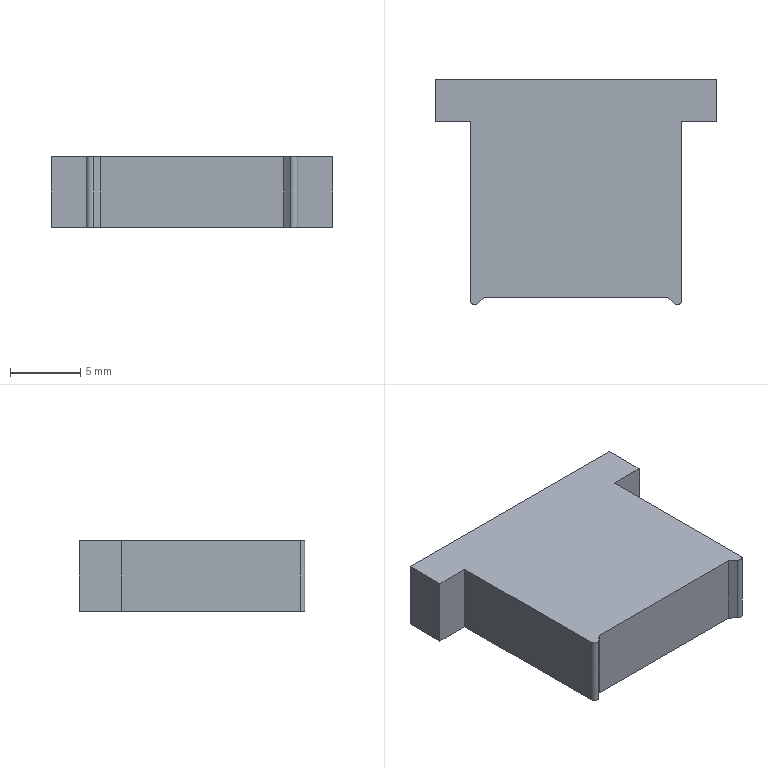Part | STEP file | iron shell positioning insert-1 | 1 solid | 17 faces | box 20 x 16.011 x 5 mm | volume 1177 mm3 | plane 11 | cylinder 6 | commonest cylinder face diameters 0.6 x2 4.5 x2 20.6 x2
STEP:
#1=CARTESIAN_POINT('',(0.,0.,0.));
#2=DIRECTION('',(0.,0.,1.));
#3=DIRECTION('',(1.,0.,0.));
#4=AXIS2_PLACEMENT_3D('',#1,#2,#3);
#5=CARTESIAN_POINT('',(-2.25,5.75,2.5));
#6=VERTEX_POINT('',#5);
#7=CARTESIAN_POINT('',(-2.25,9.75,2.5));
#8=VERTEX_POINT('',#7);
#9=CARTESIAN_POINT('',(-2.25,5.75,2.5));
#10=DIRECTION('',(0.,1.,0.));
#11=VECTOR('',#10,1.);
#12=LINE('',#9,#11);
#13=CARTESIAN_POINT('',(0.,5.75,2.5));
#14=DIRECTION('',(0.,1.,0.));
#15=DIRECTION('',(-1.,0.,0.));
#16=AXIS2_PLACEMENT_3D('',#13,#14,#15);
#17=CYLINDRICAL_SURFACE('',#16,2.25);
#18=CARTESIAN_POINT('',(6.283,0.));
#19=DIRECTION('',(0.,1.));
#20=VECTOR('',#19,1.);
#21=LINE('',#18,#20);
#22=(GEOMETRIC_REPRESENTATION_CONTEXT(2)PARAMETRIC_REPRESENTATION_CONTEXT()REPRESENTATION_CONTEXT('',''));
#23=DEFINITIONAL_REPRESENTATION('',(#21),#22);
#24=PCURVE('',#17,#23);
#25=CARTESIAN_POINT('',(0.,5.75,2.5));
#26=DIRECTION('',(0.,1.,0.));
#27=DIRECTION('',(-1.,0.,0.));
#28=AXIS2_PLACEMENT_3D('',#25,#26,#27);
#29=CYLINDRICAL_SURFACE('',#28,2.25);
#30=CARTESIAN_POINT('',(0.,0.));
#31=DIRECTION('',(0.,1.));
#32=VECTOR('',#31,1.);
#33=LINE('',#30,#32);
#34=(GEOMETRIC_REPRESENTATION_CONTEXT(2)PARAMETRIC_REPRESENTATION_CONTEXT()REPRESENTATION_CONTEXT('',''));
#35=DEFINITIONAL_REPRESENTATION('',(#33),#34);
#36=PCURVE('',#29,#35);
#37=SURFACE_CURVE('',#12,(#24,#36),.PCURVE_S1.);
#38=EDGE_CURVE('',#6,#8,#37,.T.);
#39=ORIENTED_EDGE('',*,*,#38,.T.);
#40=CARTESIAN_POINT('',(2.25,9.75,2.5));
#41=VERTEX_POINT('',#40);
#42=CARTESIAN_POINT('',(0.,9.75,2.5));
#43=DIRECTION('',(0.,1.,0.));
#44=DIRECTION('',(-1.,0.,0.));
#45=AXIS2_PLACEMENT_3D('',#42,#43,#44);
#46=CIRCLE('',#45,2.25);
#47=CARTESIAN_POINT('',(0.,4.));
#48=DIRECTION('',(1.,0.));
#49=VECTOR('',#48,1.);
#50=LINE('',#47,#49);
#51=(GEOMETRIC_REPRESENTATION_CONTEXT(2)PARAMETRIC_REPRESENTATION_CONTEXT()REPRESENTATION_CONTEXT('',''));
#52=DEFINITIONAL_REPRESENTATION('',(#50),#51);
#53=PCURVE('',#17,#52);
#54=CARTESIAN_POINT('',(-10.,9.75,5.));
#55=DIRECTION('',(0.,-1.,0.));
#56=DIRECTION('',(0.,0.,-1.));
#57=AXIS2_PLACEMENT_3D('',#54,#55,#56);
#58=PLANE('',#57);
#59=CARTESIAN_POINT('',(2.5,7.75));
#60=CARTESIAN_POINT('',(-1.397,7.75));
#61=CARTESIAN_POINT('',(0.5514,11.125));
#62=CARTESIAN_POINT('',(2.5,14.5));
#63=CARTESIAN_POINT('',(4.449,11.125));
#64=CARTESIAN_POINT('',(6.397,7.75));
#65=CARTESIAN_POINT('',(2.5,7.75));
#66=(BOUNDED_CURVE()B_SPLINE_CURVE(2,(#59,#60,#61,#62,#63,#64,#65),.UNSPECIFIED.,.T.,.F.)B_SPLINE_CURVE_WITH_KNOTS((1,2,2,2,2,1),(-2.094,0.,2.094,4.189,6.283,8.378),.UNSPECIFIED.)CURVE()GEOMETRIC_REPRESENTATION_ITEM()RATIONAL_B_SPLINE_CURVE((1.,0.5,1.,0.5,1.,0.5,1.))REPRESENTATION_ITEM(''));
#67=(GEOMETRIC_REPRESENTATION_CONTEXT(2)PARAMETRIC_REPRESENTATION_CONTEXT()REPRESENTATION_CONTEXT('',''));
#68=DEFINITIONAL_REPRESENTATION('',(#66),#67);
#69=PCURVE('',#58,#68);
#70=SURFACE_CURVE('',#46,(#53,#69),.PCURVE_S1.);
#71=EDGE_CURVE('',#41,#8,#70,.T.);
#72=ORIENTED_EDGE('',*,*,#71,.F.);
#73=CARTESIAN_POINT('',(2.25,5.75,2.5));
#74=VERTEX_POINT('',#73);
#75=CARTESIAN_POINT('',(2.25,5.75,2.5));
#76=DIRECTION('',(0.,1.,0.));
#77=VECTOR('',#76,1.);
#78=LINE('',#75,#77);
#79=CARTESIAN_POINT('',(3.142,0.));
#80=DIRECTION('',(0.,1.));
#81=VECTOR('',#80,1.);
#82=LINE('',#79,#81);
#83=(GEOMETRIC_REPRESENTATION_CONTEXT(2)PARAMETRIC_REPRESENTATION_CONTEXT()REPRESENTATION_CONTEXT('',''));
#84=DEFINITIONAL_REPRESENTATION('',(#82),#83);
#85=PCURVE('',#17,#84);
#86=CARTESIAN_POINT('',(3.142,0.));
#87=DIRECTION('',(0.,1.));
#88=VECTOR('',#87,1.);
#89=LINE('',#86,#88);
#90=(GEOMETRIC_REPRESENTATION_CONTEXT(2)PARAMETRIC_REPRESENTATION_CONTEXT()REPRESENTATION_CONTEXT('',''));
#91=DEFINITIONAL_REPRESENTATION('',(#89),#90);
#92=PCURVE('',#29,#91);
#93=SURFACE_CURVE('',#78,(#85,#92),.PCURVE_S1.);
#94=EDGE_CURVE('',#74,#41,#93,.T.);
#95=ORIENTED_EDGE('',*,*,#94,.F.);
#96=CARTESIAN_POINT('',(0.,5.75,2.5));
#97=DIRECTION('',(0.,1.,0.));
#98=DIRECTION('',(-1.,0.,0.));
#99=AXIS2_PLACEMENT_3D('',#96,#97,#98);
#100=CIRCLE('',#99,2.25);
#101=CARTESIAN_POINT('',(0.,0.));
#102=DIRECTION('',(1.,0.));
#103=VECTOR('',#102,1.);
#104=LINE('',#101,#103);
#105=(GEOMETRIC_REPRESENTATION_CONTEXT(2)PARAMETRIC_REPRESENTATION_CONTEXT()REPRESENTATION_CONTEXT('',''));
#106=DEFINITIONAL_REPRESENTATION('',(#104),#105);
#107=PCURVE('',#17,#106);
#108=CARTESIAN_POINT('',(0.,5.75,2.5));
#109=DIRECTION('',(0.,1.,0.));
#110=DIRECTION('',(-1.,0.,0.));
#111=AXIS2_PLACEMENT_3D('',#108,#109,#110);
#112=PLANE('',#111);
#113=CARTESIAN_POINT('',(0.,0.));
#114=DIRECTION('',(1.,0.));
#115=AXIS2_PLACEMENT_2D('',#113,#114);
#116=CIRCLE('',#115,2.25);
#117=(GEOMETRIC_REPRESENTATION_CONTEXT(2)PARAMETRIC_REPRESENTATION_CONTEXT()REPRESENTATION_CONTEXT('',''));
#118=DEFINITIONAL_REPRESENTATION('',(#116),#117);
#119=PCURVE('',#112,#118);
#120=SURFACE_CURVE('',#100,(#107,#119),.PCURVE_S1.);
#121=EDGE_CURVE('',#74,#6,#120,.T.);
#122=ORIENTED_EDGE('',*,*,#121,.T.);
#123=EDGE_LOOP('',(#39,#72,#95,#122));
#124=FACE_BOUND('',#123,.F.);
#125=ADVANCED_FACE('',(#124),#17,.F.);
#126=CARTESIAN_POINT('',(-10.,6.75,0.));
#127=VERTEX_POINT('',#126);
#128=CARTESIAN_POINT('',(-7.5,6.75,0.));
#129=VERTEX_POINT('',#128);
#130=CARTESIAN_POINT('',(-10.,6.75,0.));
#131=DIRECTION('',(1.,0.,0.));
#132=VECTOR('',#131,1.);
#133=LINE('',#130,#132);
#134=CARTESIAN_POINT('',(-10.,6.75,5.));
#135=DIRECTION('',(0.,1.,0.));
#136=DIRECTION('',(-1.,0.,0.));
#137=AXIS2_PLACEMENT_3D('',#134,#135,#136);
#138=PLANE('',#137);
#139=CARTESIAN_POINT('',(0.,-5.));
#140=DIRECTION('',(-1.,0.));
#141=VECTOR('',#140,1.);
#142=LINE('',#139,#141);
#143=(GEOMETRIC_REPRESENTATION_CONTEXT(2)PARAMETRIC_REPRESENTATION_CONTEXT()REPRESENTATION_CONTEXT('',''));
#144=DEFINITIONAL_REPRESENTATION('',(#142),#143);
#145=PCURVE('',#138,#144);
#146=CARTESIAN_POINT('',(-7.2,-5.961,0.));
#147=DIRECTION('',(0.,0.,1.));
#148=DIRECTION('',(1.,0.,0.));
#149=AXIS2_PLACEMENT_3D('',#146,#147,#148);
#150=PLANE('',#149);
#151=CARTESIAN_POINT('',(-2.8,12.711));
#152=DIRECTION('',(1.,0.));
#153=VECTOR('',#152,1.);
#154=LINE('',#151,#153);
#155=(GEOMETRIC_REPRESENTATION_CONTEXT(2)PARAMETRIC_REPRESENTATION_CONTEXT()REPRESENTATION_CONTEXT('',''));
#156=DEFINITIONAL_REPRESENTATION('',(#154),#155);
#157=PCURVE('',#150,#156);
#158=SURFACE_CURVE('',#133,(#145,#157),.PCURVE_S1.);
#159=EDGE_CURVE('',#127,#129,#158,.T.);
#160=ORIENTED_EDGE('',*,*,#159,.T.);
#161=CARTESIAN_POINT('',(-7.5,6.75,5.));
#162=VERTEX_POINT('',#161);
#163=CARTESIAN_POINT('',(-7.5,6.75,5.));
#164=DIRECTION('',(0.,0.,-1.));
#165=VECTOR('',#164,1.);
#166=LINE('',#163,#165);
#167=CARTESIAN_POINT('',(-2.5,0.));
#168=DIRECTION('',(0.,-1.));
#169=VECTOR('',#168,1.);
#170=LINE('',#167,#169);
#171=(GEOMETRIC_REPRESENTATION_CONTEXT(2)PARAMETRIC_REPRESENTATION_CONTEXT()REPRESENTATION_CONTEXT('',''));
#172=DEFINITIONAL_REPRESENTATION('',(#170),#171);
#173=PCURVE('',#138,#172);
#174=CARTESIAN_POINT('',(-7.5,6.75,5.));
#175=DIRECTION('',(1.,0.,0.));
#176=DIRECTION('',(0.,0.,-1.));
#177=AXIS2_PLACEMENT_3D('',#174,#175,#176);
#178=PLANE('',#177);
#179=CARTESIAN_POINT('',(0.,0.));
#180=DIRECTION('',(1.,0.));
#181=VECTOR('',#180,1.);
#182=LINE('',#179,#181);
#183=(GEOMETRIC_REPRESENTATION_CONTEXT(2)PARAMETRIC_REPRESENTATION_CONTEXT()REPRESENTATION_CONTEXT('',''));
#184=DEFINITIONAL_REPRESENTATION('',(#182),#183);
#185=PCURVE('',#178,#184);
#186=SURFACE_CURVE('',#166,(#173,#185),.PCURVE_S1.);
#187=EDGE_CURVE('',#162,#129,#186,.T.);
#188=ORIENTED_EDGE('',*,*,#187,.F.);
#189=CARTESIAN_POINT('',(-10.,6.75,5.));
#190=VERTEX_POINT('',#189);
#191=CARTESIAN_POINT('',(-10.,6.75,5.));
#192=DIRECTION('',(1.,0.,0.));
#193=VECTOR('',#192,1.);
#194=LINE('',#191,#193);
#195=CARTESIAN_POINT('',(0.,0.));
#196=DIRECTION('',(-1.,0.));
#197=VECTOR('',#196,1.);
#198=LINE('',#195,#197);
#199=(GEOMETRIC_REPRESENTATION_CONTEXT(2)PARAMETRIC_REPRESENTATION_CONTEXT()REPRESENTATION_CONTEXT('',''));
#200=DEFINITIONAL_REPRESENTATION('',(#198),#199);
#201=PCURVE('',#138,#200);
#202=CARTESIAN_POINT('',(-7.2,-5.961,5.));
#203=DIRECTION('',(0.,0.,1.));
#204=DIRECTION('',(1.,0.,0.));
#205=AXIS2_PLACEMENT_3D('',#202,#203,#204);
#206=PLANE('',#205);
#207=CARTESIAN_POINT('',(-2.8,12.711));
#208=DIRECTION('',(1.,0.));
#209=VECTOR('',#208,1.);
#210=LINE('',#207,#209);
#211=(GEOMETRIC_REPRESENTATION_CONTEXT(2)PARAMETRIC_REPRESENTATION_CONTEXT()REPRESENTATION_CONTEXT('',''));
#212=DEFINITIONAL_REPRESENTATION('',(#210),#211);
#213=PCURVE('',#206,#212);
#214=SURFACE_CURVE('',#194,(#201,#213),.PCURVE_S1.);
#215=EDGE_CURVE('',#190,#162,#214,.T.);
#216=ORIENTED_EDGE('',*,*,#215,.F.);
#217=CARTESIAN_POINT('',(-10.,6.75,5.));
#218=DIRECTION('',(0.,0.,-1.));
#219=VECTOR('',#218,1.);
#220=LINE('',#217,#219);
#221=CARTESIAN_POINT('',(0.,0.));
#222=DIRECTION('',(0.,-1.));
#223=VECTOR('',#222,1.);
#224=LINE('',#221,#223);
#225=(GEOMETRIC_REPRESENTATION_CONTEXT(2)PARAMETRIC_REPRESENTATION_CONTEXT()REPRESENTATION_CONTEXT('',''));
#226=DEFINITIONAL_REPRESENTATION('',(#224),#225);
#227=PCURVE('',#138,#226);
#228=CARTESIAN_POINT('',(-10.,9.75,5.));
#229=DIRECTION('',(1.,0.,0.));
#230=DIRECTION('',(0.,1.,0.));
#231=AXIS2_PLACEMENT_3D('',#228,#229,#230);
#232=PLANE('',#231);
#233=CARTESIAN_POINT('',(-3.,0.));
#234=DIRECTION('',(0.,-1.));
#235=VECTOR('',#234,1.);
#236=LINE('',#233,#235);
#237=(GEOMETRIC_REPRESENTATION_CONTEXT(2)PARAMETRIC_REPRESENTATION_CONTEXT()REPRESENTATION_CONTEXT('',''));
#238=DEFINITIONAL_REPRESENTATION('',(#236),#237);
#239=PCURVE('',#232,#238);
#240=SURFACE_CURVE('',#220,(#227,#239),.PCURVE_S1.);
#241=EDGE_CURVE('',#190,#127,#240,.T.);
#242=ORIENTED_EDGE('',*,*,#241,.T.);
#243=EDGE_LOOP('',(#160,#188,#216,#242));
#244=FACE_BOUND('',#243,.T.);
#245=ADVANCED_FACE('',(#244),#138,.F.);
#246=CARTESIAN_POINT('',(-7.5,-5.961,0.));
#247=VERTEX_POINT('',#246);
#248=CARTESIAN_POINT('',(-7.5,6.75,0.));
#249=DIRECTION('',(0.,-1.,0.));
#250=VECTOR('',#249,1.);
#251=LINE('',#248,#250);
#252=CARTESIAN_POINT('',(5.,0.));
#253=DIRECTION('',(0.,-1.));
#254=VECTOR('',#253,1.);
#255=LINE('',#252,#254);
#256=(GEOMETRIC_REPRESENTATION_CONTEXT(2)PARAMETRIC_REPRESENTATION_CONTEXT()REPRESENTATION_CONTEXT('',''));
#257=DEFINITIONAL_REPRESENTATION('',(#255),#256);
#258=PCURVE('',#178,#257);
#259=CARTESIAN_POINT('',(-0.3,12.711));
#260=DIRECTION('',(0.,-1.));
#261=VECTOR('',#260,1.);
#262=LINE('',#259,#261);
#263=(GEOMETRIC_REPRESENTATION_CONTEXT(2)PARAMETRIC_REPRESENTATION_CONTEXT()REPRESENTATION_CONTEXT('',''));
#264=DEFINITIONAL_REPRESENTATION('',(#262),#263);
#265=PCURVE('',#150,#264);
#266=SURFACE_CURVE('',#251,(#258,#265),.PCURVE_S1.);
#267=EDGE_CURVE('',#129,#247,#266,.T.);
#268=ORIENTED_EDGE('',*,*,#267,.T.);
#269=CARTESIAN_POINT('',(-7.5,-5.961,5.));
#270=VERTEX_POINT('',#269);
#271=CARTESIAN_POINT('',(-7.5,-5.961,5.));
#272=DIRECTION('',(0.,0.,-1.));
#273=VECTOR('',#272,1.);
#274=LINE('',#271,#273);
#275=CARTESIAN_POINT('',(0.,-12.711));
#276=DIRECTION('',(1.,0.));
#277=VECTOR('',#276,1.);
#278=LINE('',#275,#277);
#279=(GEOMETRIC_REPRESENTATION_CONTEXT(2)PARAMETRIC_REPRESENTATION_CONTEXT()REPRESENTATION_CONTEXT('',''));
#280=DEFINITIONAL_REPRESENTATION('',(#278),#279);
#281=PCURVE('',#178,#280);
#282=CARTESIAN_POINT('',(-7.2,-5.961,5.));
#283=DIRECTION('',(0.,0.,-1.));
#284=DIRECTION('',(-1.,0.,0.));
#285=AXIS2_PLACEMENT_3D('',#282,#283,#284);
#286=CYLINDRICAL_SURFACE('',#285,0.3);
#287=CARTESIAN_POINT('',(6.283,0.));
#288=DIRECTION('',(0.,1.));
#289=VECTOR('',#288,1.);
#290=LINE('',#287,#289);
#291=(GEOMETRIC_REPRESENTATION_CONTEXT(2)PARAMETRIC_REPRESENTATION_CONTEXT()REPRESENTATION_CONTEXT('',''));
#292=DEFINITIONAL_REPRESENTATION('',(#290),#291);
#293=PCURVE('',#286,#292);
#294=SURFACE_CURVE('',#274,(#281,#293),.PCURVE_S1.);
#295=EDGE_CURVE('',#270,#247,#294,.T.);
#296=ORIENTED_EDGE('',*,*,#295,.F.);
#297=CARTESIAN_POINT('',(-7.5,6.75,5.));
#298=DIRECTION('',(0.,-1.,0.));
#299=VECTOR('',#298,1.);
#300=LINE('',#297,#299);
#301=CARTESIAN_POINT('',(0.,0.));
#302=DIRECTION('',(0.,-1.));
#303=VECTOR('',#302,1.);
#304=LINE('',#301,#303);
#305=(GEOMETRIC_REPRESENTATION_CONTEXT(2)PARAMETRIC_REPRESENTATION_CONTEXT()REPRESENTATION_CONTEXT('',''));
#306=DEFINITIONAL_REPRESENTATION('',(#304),#305);
#307=PCURVE('',#178,#306);
#308=CARTESIAN_POINT('',(-0.3,12.711));
#309=DIRECTION('',(0.,-1.));
#310=VECTOR('',#309,1.);
#311=LINE('',#308,#310);
#312=(GEOMETRIC_REPRESENTATION_CONTEXT(2)PARAMETRIC_REPRESENTATION_CONTEXT()REPRESENTATION_CONTEXT('',''));
#313=DEFINITIONAL_REPRESENTATION('',(#311),#312);
#314=PCURVE('',#206,#313);
#315=SURFACE_CURVE('',#300,(#307,#314),.PCURVE_S1.);
#316=EDGE_CURVE('',#162,#270,#315,.T.);
#317=ORIENTED_EDGE('',*,*,#316,.F.);
#318=ORIENTED_EDGE('',*,*,#187,.T.);
#319=EDGE_LOOP('',(#268,#296,#317,#318));
#320=FACE_BOUND('',#319,.T.);
#321=ADVANCED_FACE('',(#320),#178,.F.);
#322=CARTESIAN_POINT('',(-6.996,-6.181,0.));
#323=VERTEX_POINT('',#322);
#324=CARTESIAN_POINT('',(-7.2,-5.961,0.));
#325=DIRECTION('',(0.,0.,1.));
#326=DIRECTION('',(1.,0.,0.));
#327=AXIS2_PLACEMENT_3D('',#324,#325,#326);
#328=CIRCLE('',#327,0.3);
#329=CARTESIAN_POINT('',(9.425,5.));
#330=DIRECTION('',(-1.,0.));
#331=VECTOR('',#330,1.);
#332=LINE('',#329,#331);
#333=(GEOMETRIC_REPRESENTATION_CONTEXT(2)PARAMETRIC_REPRESENTATION_CONTEXT()REPRESENTATION_CONTEXT('',''));
#334=DEFINITIONAL_REPRESENTATION('',(#332),#333);
#335=PCURVE('',#286,#334);
#336=CARTESIAN_POINT('',(0.,0.));
#337=DIRECTION('',(1.,0.));
#338=AXIS2_PLACEMENT_2D('',#336,#337);
#339=CIRCLE('',#338,0.3);
#340=(GEOMETRIC_REPRESENTATION_CONTEXT(2)PARAMETRIC_REPRESENTATION_CONTEXT()REPRESENTATION_CONTEXT('',''));
#341=DEFINITIONAL_REPRESENTATION('',(#339),#340);
#342=PCURVE('',#150,#341);
#343=SURFACE_CURVE('',#328,(#335,#342),.PCURVE_S1.);
#344=EDGE_CURVE('',#247,#323,#343,.T.);
#345=ORIENTED_EDGE('',*,*,#344,.T.);
#346=CARTESIAN_POINT('',(-6.996,-6.181,5.));
#347=VERTEX_POINT('',#346);
#348=CARTESIAN_POINT('',(-6.996,-6.181,5.));
#349=DIRECTION('',(0.,0.,-1.));
#350=VECTOR('',#349,1.);
#351=LINE('',#348,#350);
#352=CARTESIAN_POINT('',(3.966,0.));
#353=DIRECTION('',(0.,1.));
#354=VECTOR('',#353,1.);
#355=LINE('',#352,#354);
#356=(GEOMETRIC_REPRESENTATION_CONTEXT(2)PARAMETRIC_REPRESENTATION_CONTEXT()REPRESENTATION_CONTEXT('',''));
#357=DEFINITIONAL_REPRESENTATION('',(#355),#356);
#358=PCURVE('',#286,#357);
#359=CARTESIAN_POINT('',(0.,-13.74,5.));
#360=DIRECTION('',(0.,0.,-1.));
#361=DIRECTION('',(-1.,0.,0.));
#362=AXIS2_PLACEMENT_3D('',#359,#360,#361);
#363=CYLINDRICAL_SURFACE('',#362,10.3);
#364=CARTESIAN_POINT('',(0.8241,0.));
#365=DIRECTION('',(0.,1.));
#366=VECTOR('',#365,1.);
#367=LINE('',#364,#366);
#368=(GEOMETRIC_REPRESENTATION_CONTEXT(2)PARAMETRIC_REPRESENTATION_CONTEXT()REPRESENTATION_CONTEXT('',''));
#369=DEFINITIONAL_REPRESENTATION('',(#367),#368);
#370=PCURVE('',#363,#369);
#371=SURFACE_CURVE('',#351,(#358,#370),.PCURVE_S1.);
#372=EDGE_CURVE('',#347,#323,#371,.T.);
#373=ORIENTED_EDGE('',*,*,#372,.F.);
#374=CARTESIAN_POINT('',(-7.2,-5.961,5.));
#375=DIRECTION('',(0.,0.,1.));
#376=DIRECTION('',(1.,0.,0.));
#377=AXIS2_PLACEMENT_3D('',#374,#375,#376);
#378=CIRCLE('',#377,0.3);
#379=CARTESIAN_POINT('',(9.425,0.));
#380=DIRECTION('',(-1.,0.));
#381=VECTOR('',#380,1.);
#382=LINE('',#379,#381);
#383=(GEOMETRIC_REPRESENTATION_CONTEXT(2)PARAMETRIC_REPRESENTATION_CONTEXT()REPRESENTATION_CONTEXT('',''));
#384=DEFINITIONAL_REPRESENTATION('',(#382),#383);
#385=PCURVE('',#286,#384);
#386=CARTESIAN_POINT('',(0.,0.));
#387=DIRECTION('',(1.,0.));
#388=AXIS2_PLACEMENT_2D('',#386,#387);
#389=CIRCLE('',#388,0.3);
#390=(GEOMETRIC_REPRESENTATION_CONTEXT(2)PARAMETRIC_REPRESENTATION_CONTEXT()REPRESENTATION_CONTEXT('',''));
#391=DEFINITIONAL_REPRESENTATION('',(#389),#390);
#392=PCURVE('',#206,#391);
#393=SURFACE_CURVE('',#378,(#385,#392),.PCURVE_S1.);
#394=EDGE_CURVE('',#270,#347,#393,.T.);
#395=ORIENTED_EDGE('',*,*,#394,.F.);
#396=ORIENTED_EDGE('',*,*,#295,.T.);
#397=EDGE_LOOP('',(#345,#373,#395,#396));
#398=FACE_BOUND('',#397,.T.);
#399=ADVANCED_FACE('',(#398),#286,.T.);
#400=ORIENTED_EDGE('',*,*,#372,.F.);
#401=CARTESIAN_POINT('',(-6.5,-5.75,5.));
#402=VERTEX_POINT('',#401);
#403=CARTESIAN_POINT('',(0.,-13.74,5.));
#404=DIRECTION('',(0.,0.,-1.));
#405=DIRECTION('',(1.,0.,0.));
#406=AXIS2_PLACEMENT_3D('',#403,#404,#405);
#407=CIRCLE('',#406,10.3);
#408=CARTESIAN_POINT('',(-3.142,0.));
#409=DIRECTION('',(1.,0.));
#410=VECTOR('',#409,1.);
#411=LINE('',#408,#410);
#412=(GEOMETRIC_REPRESENTATION_CONTEXT(2)PARAMETRIC_REPRESENTATION_CONTEXT()REPRESENTATION_CONTEXT('',''));
#413=DEFINITIONAL_REPRESENTATION('',(#411),#412);
#414=PCURVE('',#363,#413);
#415=CARTESIAN_POINT('',(17.5,-7.779));
#416=CARTESIAN_POINT('',(17.5,-25.62));
#417=CARTESIAN_POINT('',(2.05,-16.7));
#418=CARTESIAN_POINT('',(-13.4,-7.779));
#419=CARTESIAN_POINT('',(2.05,1.141));
#420=CARTESIAN_POINT('',(17.5,10.061));
#421=CARTESIAN_POINT('',(17.5,-7.779));
#422=(BOUNDED_CURVE()B_SPLINE_CURVE(2,(#415,#416,#417,#418,#419,#420,#421),.UNSPECIFIED.,.T.,.F.)B_SPLINE_CURVE_WITH_KNOTS((1,2,2,2,2,1),(-2.094,0.,2.094,4.189,6.283,8.378),.UNSPECIFIED.)CURVE()GEOMETRIC_REPRESENTATION_ITEM()RATIONAL_B_SPLINE_CURVE((1.,0.5,1.,0.5,1.,0.5,1.))REPRESENTATION_ITEM(''));
#423=(GEOMETRIC_REPRESENTATION_CONTEXT(2)PARAMETRIC_REPRESENTATION_CONTEXT()REPRESENTATION_CONTEXT('',''));
#424=DEFINITIONAL_REPRESENTATION('',(#422),#423);
#425=PCURVE('',#206,#424);
#426=SURFACE_CURVE('',#407,(#414,#425),.PCURVE_S1.);
#427=EDGE_CURVE('',#347,#402,#426,.T.);
#428=ORIENTED_EDGE('',*,*,#427,.T.);
#429=CARTESIAN_POINT('',(-6.5,-5.75,0.));
#430=VERTEX_POINT('',#429);
#431=CARTESIAN_POINT('',(-6.5,-5.75,5.));
#432=DIRECTION('',(0.,0.,-1.));
#433=VECTOR('',#432,1.);
#434=LINE('',#431,#433);
#435=CARTESIAN_POINT('',(0.8879,0.));
#436=DIRECTION('',(0.,1.));
#437=VECTOR('',#436,1.);
#438=LINE('',#435,#437);
#439=(GEOMETRIC_REPRESENTATION_CONTEXT(2)PARAMETRIC_REPRESENTATION_CONTEXT()REPRESENTATION_CONTEXT('',''));
#440=DEFINITIONAL_REPRESENTATION('',(#438),#439);
#441=PCURVE('',#363,#440);
#442=CARTESIAN_POINT('',(-6.5,-5.75,5.));
#443=DIRECTION('',(0.,1.,0.));
#444=DIRECTION('',(0.,0.,1.));
#445=AXIS2_PLACEMENT_3D('',#442,#443,#444);
#446=PLANE('',#445);
#447=CARTESIAN_POINT('',(0.,0.));
#448=DIRECTION('',(-1.,0.));
#449=VECTOR('',#448,1.);
#450=LINE('',#447,#449);
#451=(GEOMETRIC_REPRESENTATION_CONTEXT(2)PARAMETRIC_REPRESENTATION_CONTEXT()REPRESENTATION_CONTEXT('',''));
#452=DEFINITIONAL_REPRESENTATION('',(#450),#451);
#453=PCURVE('',#446,#452);
#454=SURFACE_CURVE('',#434,(#441,#453),.PCURVE_S1.);
#455=EDGE_CURVE('',#402,#430,#454,.T.);
#456=ORIENTED_EDGE('',*,*,#455,.T.);
#457=CARTESIAN_POINT('',(0.,-13.74,0.));
#458=DIRECTION('',(0.,0.,-1.));
#459=DIRECTION('',(1.,0.,0.));
#460=AXIS2_PLACEMENT_3D('',#457,#458,#459);
#461=CIRCLE('',#460,10.3);
#462=CARTESIAN_POINT('',(-3.142,5.));
#463=DIRECTION('',(1.,0.));
#464=VECTOR('',#463,1.);
#465=LINE('',#462,#464);
#466=(GEOMETRIC_REPRESENTATION_CONTEXT(2)PARAMETRIC_REPRESENTATION_CONTEXT()REPRESENTATION_CONTEXT('',''));
#467=DEFINITIONAL_REPRESENTATION('',(#465),#466);
#468=PCURVE('',#363,#467);
#469=CARTESIAN_POINT('',(17.5,-7.779));
#470=CARTESIAN_POINT('',(17.5,-25.62));
#471=CARTESIAN_POINT('',(2.05,-16.7));
#472=CARTESIAN_POINT('',(-13.4,-7.779));
#473=CARTESIAN_POINT('',(2.05,1.141));
#474=CARTESIAN_POINT('',(17.5,10.061));
#475=CARTESIAN_POINT('',(17.5,-7.779));
#476=(BOUNDED_CURVE()B_SPLINE_CURVE(2,(#469,#470,#471,#472,#473,#474,#475),.UNSPECIFIED.,.T.,.F.)B_SPLINE_CURVE_WITH_KNOTS((1,2,2,2,2,1),(-2.094,0.,2.094,4.189,6.283,8.378),.UNSPECIFIED.)CURVE()GEOMETRIC_REPRESENTATION_ITEM()RATIONAL_B_SPLINE_CURVE((1.,0.5,1.,0.5,1.,0.5,1.))REPRESENTATION_ITEM(''));
#477=(GEOMETRIC_REPRESENTATION_CONTEXT(2)PARAMETRIC_REPRESENTATION_CONTEXT()REPRESENTATION_CONTEXT('',''));
#478=DEFINITIONAL_REPRESENTATION('',(#476),#477);
#479=PCURVE('',#150,#478);
#480=SURFACE_CURVE('',#461,(#468,#479),.PCURVE_S1.);
#481=EDGE_CURVE('',#323,#430,#480,.T.);
#482=ORIENTED_EDGE('',*,*,#481,.F.);
#483=EDGE_LOOP('',(#400,#428,#456,#482));
#484=FACE_BOUND('',#483,.F.);
#485=ADVANCED_FACE('',(#484),#363,.F.);
#486=CARTESIAN_POINT('',(6.5,-5.75,0.));
#487=VERTEX_POINT('',#486);
#488=CARTESIAN_POINT('',(-6.5,-5.75,0.));
#489=DIRECTION('',(1.,0.,0.));
#490=VECTOR('',#489,1.);
#491=LINE('',#488,#490);
#492=CARTESIAN_POINT('',(-5.,0.));
#493=DIRECTION('',(0.,1.));
#494=VECTOR('',#493,1.);
#495=LINE('',#492,#494);
#496=(GEOMETRIC_REPRESENTATION_CONTEXT(2)PARAMETRIC_REPRESENTATION_CONTEXT()REPRESENTATION_CONTEXT('',''));
#497=DEFINITIONAL_REPRESENTATION('',(#495),#496);
#498=PCURVE('',#446,#497);
#499=CARTESIAN_POINT('',(0.7,0.2105));
#500=DIRECTION('',(1.,0.));
#501=VECTOR('',#500,1.);
#502=LINE('',#499,#501);
#503=(GEOMETRIC_REPRESENTATION_CONTEXT(2)PARAMETRIC_REPRESENTATION_CONTEXT()REPRESENTATION_CONTEXT('',''));
#504=DEFINITIONAL_REPRESENTATION('',(#502),#503);
#505=PCURVE('',#150,#504);
#506=SURFACE_CURVE('',#491,(#498,#505),.PCURVE_S1.);
#507=EDGE_CURVE('',#430,#487,#506,.T.);
#508=ORIENTED_EDGE('',*,*,#507,.T.);
#509=CARTESIAN_POINT('',(6.5,-5.75,5.));
#510=VERTEX_POINT('',#509);
#511=CARTESIAN_POINT('',(6.5,-5.75,5.));
#512=DIRECTION('',(0.,0.,-1.));
#513=VECTOR('',#512,1.);
#514=LINE('',#511,#513);
#515=CARTESIAN_POINT('',(0.,13.));
#516=DIRECTION('',(-1.,0.));
#517=VECTOR('',#516,1.);
#518=LINE('',#515,#517);
#519=(GEOMETRIC_REPRESENTATION_CONTEXT(2)PARAMETRIC_REPRESENTATION_CONTEXT()REPRESENTATION_CONTEXT('',''));
#520=DEFINITIONAL_REPRESENTATION('',(#518),#519);
#521=PCURVE('',#446,#520);
#522=CARTESIAN_POINT('',(0.,-13.74,5.));
#523=DIRECTION('',(0.,0.,-1.));
#524=DIRECTION('',(-1.,0.,0.));
#525=AXIS2_PLACEMENT_3D('',#522,#523,#524);
#526=CYLINDRICAL_SURFACE('',#525,10.3);
#527=CARTESIAN_POINT('',(2.254,0.));
#528=DIRECTION('',(0.,1.));
#529=VECTOR('',#528,1.);
#530=LINE('',#527,#529);
#531=(GEOMETRIC_REPRESENTATION_CONTEXT(2)PARAMETRIC_REPRESENTATION_CONTEXT()REPRESENTATION_CONTEXT('',''));
#532=DEFINITIONAL_REPRESENTATION('',(#530),#531);
#533=PCURVE('',#526,#532);
#534=SURFACE_CURVE('',#514,(#521,#533),.PCURVE_S1.);
#535=EDGE_CURVE('',#510,#487,#534,.T.);
#536=ORIENTED_EDGE('',*,*,#535,.F.);
#537=CARTESIAN_POINT('',(-6.5,-5.75,5.));
#538=DIRECTION('',(1.,0.,0.));
#539=VECTOR('',#538,1.);
#540=LINE('',#537,#539);
#541=CARTESIAN_POINT('',(0.,0.));
#542=DIRECTION('',(0.,1.));
#543=VECTOR('',#542,1.);
#544=LINE('',#541,#543);
#545=(GEOMETRIC_REPRESENTATION_CONTEXT(2)PARAMETRIC_REPRESENTATION_CONTEXT()REPRESENTATION_CONTEXT('',''));
#546=DEFINITIONAL_REPRESENTATION('',(#544),#545);
#547=PCURVE('',#446,#546);
#548=CARTESIAN_POINT('',(0.7,0.2105));
#549=DIRECTION('',(1.,0.));
#550=VECTOR('',#549,1.);
#551=LINE('',#548,#550);
#552=(GEOMETRIC_REPRESENTATION_CONTEXT(2)PARAMETRIC_REPRESENTATION_CONTEXT()REPRESENTATION_CONTEXT('',''));
#553=DEFINITIONAL_REPRESENTATION('',(#551),#552);
#554=PCURVE('',#206,#553);
#555=SURFACE_CURVE('',#540,(#547,#554),.PCURVE_S1.);
#556=EDGE_CURVE('',#402,#510,#555,.T.);
#557=ORIENTED_EDGE('',*,*,#556,.F.);
#558=ORIENTED_EDGE('',*,*,#455,.T.);
#559=EDGE_LOOP('',(#508,#536,#557,#558));
#560=FACE_BOUND('',#559,.T.);
#561=ADVANCED_FACE('',(#560),#446,.F.);
#562=ORIENTED_EDGE('',*,*,#535,.F.);
#563=CARTESIAN_POINT('',(6.996,-6.181,5.));
#564=VERTEX_POINT('',#563);
#565=CARTESIAN_POINT('',(0.,-13.74,5.));
#566=DIRECTION('',(0.,0.,-1.));
#567=DIRECTION('',(1.,0.,0.));
#568=AXIS2_PLACEMENT_3D('',#565,#566,#567);
#569=CIRCLE('',#568,10.3);
#570=CARTESIAN_POINT('',(-3.142,0.));
#571=DIRECTION('',(1.,0.));
#572=VECTOR('',#571,1.);
#573=LINE('',#570,#572);
#574=(GEOMETRIC_REPRESENTATION_CONTEXT(2)PARAMETRIC_REPRESENTATION_CONTEXT()REPRESENTATION_CONTEXT('',''));
#575=DEFINITIONAL_REPRESENTATION('',(#573),#574);
#576=PCURVE('',#526,#575);
#577=CARTESIAN_POINT('',(17.5,-7.779));
#578=CARTESIAN_POINT('',(17.5,-25.62));
#579=CARTESIAN_POINT('',(2.05,-16.7));
#580=CARTESIAN_POINT('',(-13.4,-7.779));
#581=CARTESIAN_POINT('',(2.05,1.141));
#582=CARTESIAN_POINT('',(17.5,10.061));
#583=CARTESIAN_POINT('',(17.5,-7.779));
#584=(BOUNDED_CURVE()B_SPLINE_CURVE(2,(#577,#578,#579,#580,#581,#582,#583),.UNSPECIFIED.,.T.,.F.)B_SPLINE_CURVE_WITH_KNOTS((1,2,2,2,2,1),(-2.094,0.,2.094,4.189,6.283,8.378),.UNSPECIFIED.)CURVE()GEOMETRIC_REPRESENTATION_ITEM()RATIONAL_B_SPLINE_CURVE((1.,0.5,1.,0.5,1.,0.5,1.))REPRESENTATION_ITEM(''));
#585=(GEOMETRIC_REPRESENTATION_CONTEXT(2)PARAMETRIC_REPRESENTATION_CONTEXT()REPRESENTATION_CONTEXT('',''));
#586=DEFINITIONAL_REPRESENTATION('',(#584),#585);
#587=PCURVE('',#206,#586);
#588=SURFACE_CURVE('',#569,(#576,#587),.PCURVE_S1.);
#589=EDGE_CURVE('',#510,#564,#588,.T.);
#590=ORIENTED_EDGE('',*,*,#589,.T.);
#591=CARTESIAN_POINT('',(6.996,-6.181,0.));
#592=VERTEX_POINT('',#591);
#593=CARTESIAN_POINT('',(6.996,-6.181,5.));
#594=DIRECTION('',(0.,0.,-1.));
#595=VECTOR('',#594,1.);
#596=LINE('',#593,#595);
#597=CARTESIAN_POINT('',(2.318,0.));
#598=DIRECTION('',(0.,1.));
#599=VECTOR('',#598,1.);
#600=LINE('',#597,#599);
#601=(GEOMETRIC_REPRESENTATION_CONTEXT(2)PARAMETRIC_REPRESENTATION_CONTEXT()REPRESENTATION_CONTEXT('',''));
#602=DEFINITIONAL_REPRESENTATION('',(#600),#601);
#603=PCURVE('',#526,#602);
#604=CARTESIAN_POINT('',(7.2,-5.961,5.));
#605=DIRECTION('',(0.,0.,-1.));
#606=DIRECTION('',(-1.,0.,0.));
#607=AXIS2_PLACEMENT_3D('',#604,#605,#606);
#608=CYLINDRICAL_SURFACE('',#607,0.3);
#609=CARTESIAN_POINT('',(5.459,0.));
#610=DIRECTION('',(0.,1.));
#611=VECTOR('',#610,1.);
#612=LINE('',#609,#611);
#613=(GEOMETRIC_REPRESENTATION_CONTEXT(2)PARAMETRIC_REPRESENTATION_CONTEXT()REPRESENTATION_CONTEXT('',''));
#614=DEFINITIONAL_REPRESENTATION('',(#612),#613);
#615=PCURVE('',#608,#614);
#616=SURFACE_CURVE('',#596,(#603,#615),.PCURVE_S1.);
#617=EDGE_CURVE('',#564,#592,#616,.T.);
#618=ORIENTED_EDGE('',*,*,#617,.T.);
#619=CARTESIAN_POINT('',(0.,-13.74,0.));
#620=DIRECTION('',(0.,0.,-1.));
#621=DIRECTION('',(1.,0.,0.));
#622=AXIS2_PLACEMENT_3D('',#619,#620,#621);
#623=CIRCLE('',#622,10.3);
#624=CARTESIAN_POINT('',(-3.142,5.));
#625=DIRECTION('',(1.,0.));
#626=VECTOR('',#625,1.);
#627=LINE('',#624,#626);
#628=(GEOMETRIC_REPRESENTATION_CONTEXT(2)PARAMETRIC_REPRESENTATION_CONTEXT()REPRESENTATION_CONTEXT('',''));
#629=DEFINITIONAL_REPRESENTATION('',(#627),#628);
#630=PCURVE('',#526,#629);
#631=CARTESIAN_POINT('',(17.5,-7.779));
#632=CARTESIAN_POINT('',(17.5,-25.62));
#633=CARTESIAN_POINT('',(2.05,-16.7));
#634=CARTESIAN_POINT('',(-13.4,-7.779));
#635=CARTESIAN_POINT('',(2.05,1.141));
#636=CARTESIAN_POINT('',(17.5,10.061));
#637=CARTESIAN_POINT('',(17.5,-7.779));
#638=(BOUNDED_CURVE()B_SPLINE_CURVE(2,(#631,#632,#633,#634,#635,#636,#637),.UNSPECIFIED.,.T.,.F.)B_SPLINE_CURVE_WITH_KNOTS((1,2,2,2,2,1),(-2.094,0.,2.094,4.189,6.283,8.378),.UNSPECIFIED.)CURVE()GEOMETRIC_REPRESENTATION_ITEM()RATIONAL_B_SPLINE_CURVE((1.,0.5,1.,0.5,1.,0.5,1.))REPRESENTATION_ITEM(''));
#639=(GEOMETRIC_REPRESENTATION_CONTEXT(2)PARAMETRIC_REPRESENTATION_CONTEXT()REPRESENTATION_CONTEXT('',''));
#640=DEFINITIONAL_REPRESENTATION('',(#638),#639);
#641=PCURVE('',#150,#640);
#642=SURFACE_CURVE('',#623,(#630,#641),.PCURVE_S1.);
#643=EDGE_CURVE('',#487,#592,#642,.T.);
#644=ORIENTED_EDGE('',*,*,#643,.F.);
#645=EDGE_LOOP('',(#562,#590,#618,#644));
#646=FACE_BOUND('',#645,.F.);
#647=ADVANCED_FACE('',(#646),#526,.F.);
#648=CARTESIAN_POINT('',(7.5,-5.961,0.));
#649=VERTEX_POINT('',#648);
#650=CARTESIAN_POINT('',(7.2,-5.961,0.));
#651=DIRECTION('',(0.,0.,1.));
#652=DIRECTION('',(1.,0.,0.));
#653=AXIS2_PLACEMENT_3D('',#650,#651,#652);
#654=CIRCLE('',#653,0.3);
#655=CARTESIAN_POINT('',(9.425,5.));
#656=DIRECTION('',(-1.,0.));
#657=VECTOR('',#656,1.);
#658=LINE('',#655,#657);
#659=(GEOMETRIC_REPRESENTATION_CONTEXT(2)PARAMETRIC_REPRESENTATION_CONTEXT()REPRESENTATION_CONTEXT('',''));
#660=DEFINITIONAL_REPRESENTATION('',(#658),#659);
#661=PCURVE('',#608,#660);
#662=CARTESIAN_POINT('',(14.4,0.));
#663=DIRECTION('',(1.,0.));
#664=AXIS2_PLACEMENT_2D('',#662,#663);
#665=CIRCLE('',#664,0.3);
#666=(GEOMETRIC_REPRESENTATION_CONTEXT(2)PARAMETRIC_REPRESENTATION_CONTEXT()REPRESENTATION_CONTEXT('',''));
#667=DEFINITIONAL_REPRESENTATION('',(#665),#666);
#668=PCURVE('',#150,#667);
#669=SURFACE_CURVE('',#654,(#661,#668),.PCURVE_S1.);
#670=EDGE_CURVE('',#592,#649,#669,.T.);
#671=ORIENTED_EDGE('',*,*,#670,.T.);
#672=CARTESIAN_POINT('',(7.5,-5.961,5.));
#673=VERTEX_POINT('',#672);
#674=CARTESIAN_POINT('',(7.5,-5.961,5.));
#675=DIRECTION('',(0.,0.,-1.));
#676=VECTOR('',#675,1.);
#677=LINE('',#674,#676);
#678=CARTESIAN_POINT('',(3.142,0.));
#679=DIRECTION('',(0.,1.));
#680=VECTOR('',#679,1.);
#681=LINE('',#678,#680);
#682=(GEOMETRIC_REPRESENTATION_CONTEXT(2)PARAMETRIC_REPRESENTATION_CONTEXT()REPRESENTATION_CONTEXT('',''));
#683=DEFINITIONAL_REPRESENTATION('',(#681),#682);
#684=PCURVE('',#608,#683);
#685=CARTESIAN_POINT('',(7.5,6.75,5.));
#686=DIRECTION('',(-1.,0.,0.));
#687=DIRECTION('',(0.,0.,1.));
#688=AXIS2_PLACEMENT_3D('',#685,#686,#687);
#689=PLANE('',#688);
#690=CARTESIAN_POINT('',(0.,-12.711));
#691=DIRECTION('',(-1.,0.));
#692=VECTOR('',#691,1.);
#693=LINE('',#690,#692);
#694=(GEOMETRIC_REPRESENTATION_CONTEXT(2)PARAMETRIC_REPRESENTATION_CONTEXT()REPRESENTATION_CONTEXT('',''));
#695=DEFINITIONAL_REPRESENTATION('',(#693),#694);
#696=PCURVE('',#689,#695);
#697=SURFACE_CURVE('',#677,(#684,#696),.PCURVE_S1.);
#698=EDGE_CURVE('',#673,#649,#697,.T.);
#699=ORIENTED_EDGE('',*,*,#698,.F.);
#700=CARTESIAN_POINT('',(7.2,-5.961,5.));
#701=DIRECTION('',(0.,0.,1.));
#702=DIRECTION('',(1.,0.,0.));
#703=AXIS2_PLACEMENT_3D('',#700,#701,#702);
#704=CIRCLE('',#703,0.3);
#705=CARTESIAN_POINT('',(9.425,0.));
#706=DIRECTION('',(-1.,0.));
#707=VECTOR('',#706,1.);
#708=LINE('',#705,#707);
#709=(GEOMETRIC_REPRESENTATION_CONTEXT(2)PARAMETRIC_REPRESENTATION_CONTEXT()REPRESENTATION_CONTEXT('',''));
#710=DEFINITIONAL_REPRESENTATION('',(#708),#709);
#711=PCURVE('',#608,#710);
#712=CARTESIAN_POINT('',(14.4,0.));
#713=DIRECTION('',(1.,0.));
#714=AXIS2_PLACEMENT_2D('',#712,#713);
#715=CIRCLE('',#714,0.3);
#716=(GEOMETRIC_REPRESENTATION_CONTEXT(2)PARAMETRIC_REPRESENTATION_CONTEXT()REPRESENTATION_CONTEXT('',''));
#717=DEFINITIONAL_REPRESENTATION('',(#715),#716);
#718=PCURVE('',#206,#717);
#719=SURFACE_CURVE('',#704,(#711,#718),.PCURVE_S1.);
#720=EDGE_CURVE('',#564,#673,#719,.T.);
#721=ORIENTED_EDGE('',*,*,#720,.F.);
#722=ORIENTED_EDGE('',*,*,#617,.T.);
#723=EDGE_LOOP('',(#671,#699,#721,#722));
#724=FACE_BOUND('',#723,.T.);
#725=ADVANCED_FACE('',(#724),#608,.T.);
#726=CARTESIAN_POINT('',(7.5,6.75,0.));
#727=VERTEX_POINT('',#726);
#728=CARTESIAN_POINT('',(7.5,6.75,0.));
#729=DIRECTION('',(0.,1.,0.));
#730=VECTOR('',#729,1.);
#731=LINE('',#728,#730);
#732=CARTESIAN_POINT('',(-5.,0.));
#733=DIRECTION('',(0.,1.));
#734=VECTOR('',#733,1.);
#735=LINE('',#732,#734);
#736=(GEOMETRIC_REPRESENTATION_CONTEXT(2)PARAMETRIC_REPRESENTATION_CONTEXT()REPRESENTATION_CONTEXT('',''));
#737=DEFINITIONAL_REPRESENTATION('',(#735),#736);
#738=PCURVE('',#689,#737);
#739=CARTESIAN_POINT('',(14.7,12.711));
#740=DIRECTION('',(0.,1.));
#741=VECTOR('',#740,1.);
#742=LINE('',#739,#741);
#743=(GEOMETRIC_REPRESENTATION_CONTEXT(2)PARAMETRIC_REPRESENTATION_CONTEXT()REPRESENTATION_CONTEXT('',''));
#744=DEFINITIONAL_REPRESENTATION('',(#742),#743);
#745=PCURVE('',#150,#744);
#746=SURFACE_CURVE('',#731,(#738,#745),.PCURVE_S1.);
#747=EDGE_CURVE('',#649,#727,#746,.T.);
#748=ORIENTED_EDGE('',*,*,#747,.T.);
#749=CARTESIAN_POINT('',(7.5,6.75,5.));
#750=VERTEX_POINT('',#749);
#751=CARTESIAN_POINT('',(7.5,6.75,5.));
#752=DIRECTION('',(0.,0.,-1.));
#753=VECTOR('',#752,1.);
#754=LINE('',#751,#753);
#755=CARTESIAN_POINT('',(0.,0.));
#756=DIRECTION('',(-1.,0.));
#757=VECTOR('',#756,1.);
#758=LINE('',#755,#757);
#759=(GEOMETRIC_REPRESENTATION_CONTEXT(2)PARAMETRIC_REPRESENTATION_CONTEXT()REPRESENTATION_CONTEXT('',''));
#760=DEFINITIONAL_REPRESENTATION('',(#758),#759);
#761=PCURVE('',#689,#760);
#762=CARTESIAN_POINT('',(7.5,6.75,5.));
#763=DIRECTION('',(0.,1.,0.));
#764=DIRECTION('',(-1.,0.,0.));
#765=AXIS2_PLACEMENT_3D('',#762,#763,#764);
#766=PLANE('',#765);
#767=CARTESIAN_POINT('',(0.,0.));
#768=DIRECTION('',(0.,-1.));
#769=VECTOR('',#768,1.);
#770=LINE('',#767,#769);
#771=(GEOMETRIC_REPRESENTATION_CONTEXT(2)PARAMETRIC_REPRESENTATION_CONTEXT()REPRESENTATION_CONTEXT('',''));
#772=DEFINITIONAL_REPRESENTATION('',(#770),#771);
#773=PCURVE('',#766,#772);
#774=SURFACE_CURVE('',#754,(#761,#773),.PCURVE_S1.);
#775=EDGE_CURVE('',#750,#727,#774,.T.);
#776=ORIENTED_EDGE('',*,*,#775,.F.);
#777=CARTESIAN_POINT('',(7.5,6.75,5.));
#778=DIRECTION('',(0.,1.,0.));
#779=VECTOR('',#778,1.);
#780=LINE('',#777,#779);
#781=CARTESIAN_POINT('',(0.,0.));
#782=DIRECTION('',(0.,1.));
#783=VECTOR('',#782,1.);
#784=LINE('',#781,#783);
#785=(GEOMETRIC_REPRESENTATION_CONTEXT(2)PARAMETRIC_REPRESENTATION_CONTEXT()REPRESENTATION_CONTEXT('',''));
#786=DEFINITIONAL_REPRESENTATION('',(#784),#785);
#787=PCURVE('',#689,#786);
#788=CARTESIAN_POINT('',(14.7,12.711));
#789=DIRECTION('',(0.,1.));
#790=VECTOR('',#789,1.);
#791=LINE('',#788,#790);
#792=(GEOMETRIC_REPRESENTATION_CONTEXT(2)PARAMETRIC_REPRESENTATION_CONTEXT()REPRESENTATION_CONTEXT('',''));
#793=DEFINITIONAL_REPRESENTATION('',(#791),#792);
#794=PCURVE('',#206,#793);
#795=SURFACE_CURVE('',#780,(#787,#794),.PCURVE_S1.);
#796=EDGE_CURVE('',#673,#750,#795,.T.);
#797=ORIENTED_EDGE('',*,*,#796,.F.);
#798=ORIENTED_EDGE('',*,*,#698,.T.);
#799=EDGE_LOOP('',(#748,#776,#797,#798));
#800=FACE_BOUND('',#799,.T.);
#801=ADVANCED_FACE('',(#800),#689,.F.);
#802=CARTESIAN_POINT('',(10.,6.75,0.));
#803=VERTEX_POINT('',#802);
#804=CARTESIAN_POINT('',(7.5,6.75,0.));
#805=DIRECTION('',(1.,0.,0.));
#806=VECTOR('',#805,1.);
#807=LINE('',#804,#806);
#808=CARTESIAN_POINT('',(0.,-5.));
#809=DIRECTION('',(-1.,0.));
#810=VECTOR('',#809,1.);
#811=LINE('',#808,#810);
#812=(GEOMETRIC_REPRESENTATION_CONTEXT(2)PARAMETRIC_REPRESENTATION_CONTEXT()REPRESENTATION_CONTEXT('',''));
#813=DEFINITIONAL_REPRESENTATION('',(#811),#812);
#814=PCURVE('',#766,#813);
#815=CARTESIAN_POINT('',(14.7,12.711));
#816=DIRECTION('',(1.,0.));
#817=VECTOR('',#816,1.);
#818=LINE('',#815,#817);
#819=(GEOMETRIC_REPRESENTATION_CONTEXT(2)PARAMETRIC_REPRESENTATION_CONTEXT()REPRESENTATION_CONTEXT('',''));
#820=DEFINITIONAL_REPRESENTATION('',(#818),#819);
#821=PCURVE('',#150,#820);
#822=SURFACE_CURVE('',#807,(#814,#821),.PCURVE_S1.);
#823=EDGE_CURVE('',#727,#803,#822,.T.);
#824=ORIENTED_EDGE('',*,*,#823,.T.);
#825=CARTESIAN_POINT('',(10.,6.75,5.));
#826=VERTEX_POINT('',#825);
#827=CARTESIAN_POINT('',(10.,6.75,5.));
#828=DIRECTION('',(0.,0.,-1.));
#829=VECTOR('',#828,1.);
#830=LINE('',#827,#829);
#831=CARTESIAN_POINT('',(-2.5,0.));
#832=DIRECTION('',(0.,-1.));
#833=VECTOR('',#832,1.);
#834=LINE('',#831,#833);
#835=(GEOMETRIC_REPRESENTATION_CONTEXT(2)PARAMETRIC_REPRESENTATION_CONTEXT()REPRESENTATION_CONTEXT('',''));
#836=DEFINITIONAL_REPRESENTATION('',(#834),#835);
#837=PCURVE('',#766,#836);
#838=CARTESIAN_POINT('',(10.,9.75,5.));
#839=DIRECTION('',(-1.,0.,0.));
#840=DIRECTION('',(0.,-1.,0.));
#841=AXIS2_PLACEMENT_3D('',#838,#839,#840);
#842=PLANE('',#841);
#843=CARTESIAN_POINT('',(3.,0.));
#844=DIRECTION('',(0.,-1.));
#845=VECTOR('',#844,1.);
#846=LINE('',#843,#845);
#847=(GEOMETRIC_REPRESENTATION_CONTEXT(2)PARAMETRIC_REPRESENTATION_CONTEXT()REPRESENTATION_CONTEXT('',''));
#848=DEFINITIONAL_REPRESENTATION('',(#846),#847);
#849=PCURVE('',#842,#848);
#850=SURFACE_CURVE('',#830,(#837,#849),.PCURVE_S1.);
#851=EDGE_CURVE('',#826,#803,#850,.T.);
#852=ORIENTED_EDGE('',*,*,#851,.F.);
#853=CARTESIAN_POINT('',(7.5,6.75,5.));
#854=DIRECTION('',(1.,0.,0.));
#855=VECTOR('',#854,1.);
#856=LINE('',#853,#855);
#857=CARTESIAN_POINT('',(0.,0.));
#858=DIRECTION('',(-1.,0.));
#859=VECTOR('',#858,1.);
#860=LINE('',#857,#859);
#861=(GEOMETRIC_REPRESENTATION_CONTEXT(2)PARAMETRIC_REPRESENTATION_CONTEXT()REPRESENTATION_CONTEXT('',''));
#862=DEFINITIONAL_REPRESENTATION('',(#860),#861);
#863=PCURVE('',#766,#862);
#864=CARTESIAN_POINT('',(14.7,12.711));
#865=DIRECTION('',(1.,0.));
#866=VECTOR('',#865,1.);
#867=LINE('',#864,#866);
#868=(GEOMETRIC_REPRESENTATION_CONTEXT(2)PARAMETRIC_REPRESENTATION_CONTEXT()REPRESENTATION_CONTEXT('',''));
#869=DEFINITIONAL_REPRESENTATION('',(#867),#868);
#870=PCURVE('',#206,#869);
#871=SURFACE_CURVE('',#856,(#863,#870),.PCURVE_S1.);
#872=EDGE_CURVE('',#750,#826,#871,.T.);
#873=ORIENTED_EDGE('',*,*,#872,.F.);
#874=ORIENTED_EDGE('',*,*,#775,.T.);
#875=EDGE_LOOP('',(#824,#852,#873,#874));
#876=FACE_BOUND('',#875,.T.);
#877=ADVANCED_FACE('',(#876),#766,.F.);
#878=CARTESIAN_POINT('',(10.,9.75,0.));
#879=VERTEX_POINT('',#878);
#880=CARTESIAN_POINT('',(10.,9.75,0.));
#881=DIRECTION('',(0.,1.,0.));
#882=VECTOR('',#881,1.);
#883=LINE('',#880,#882);
#884=CARTESIAN_POINT('',(0.,-5.));
#885=DIRECTION('',(-1.,0.));
#886=VECTOR('',#885,1.);
#887=LINE('',#884,#886);
#888=(GEOMETRIC_REPRESENTATION_CONTEXT(2)PARAMETRIC_REPRESENTATION_CONTEXT()REPRESENTATION_CONTEXT('',''));
#889=DEFINITIONAL_REPRESENTATION('',(#887),#888);
#890=PCURVE('',#842,#889);
#891=CARTESIAN_POINT('',(17.2,15.711));
#892=DIRECTION('',(0.,1.));
#893=VECTOR('',#892,1.);
#894=LINE('',#891,#893);
#895=(GEOMETRIC_REPRESENTATION_CONTEXT(2)PARAMETRIC_REPRESENTATION_CONTEXT()REPRESENTATION_CONTEXT('',''));
#896=DEFINITIONAL_REPRESENTATION('',(#894),#895);
#897=PCURVE('',#150,#896);
#898=SURFACE_CURVE('',#883,(#890,#897),.PCURVE_S1.);
#899=EDGE_CURVE('',#803,#879,#898,.T.);
#900=ORIENTED_EDGE('',*,*,#899,.T.);
#901=CARTESIAN_POINT('',(10.,9.75,5.));
#902=VERTEX_POINT('',#901);
#903=CARTESIAN_POINT('',(10.,9.75,5.));
#904=DIRECTION('',(0.,0.,-1.));
#905=VECTOR('',#904,1.);
#906=LINE('',#903,#905);
#907=CARTESIAN_POINT('',(0.,0.));
#908=DIRECTION('',(0.,-1.));
#909=VECTOR('',#908,1.);
#910=LINE('',#907,#909);
#911=(GEOMETRIC_REPRESENTATION_CONTEXT(2)PARAMETRIC_REPRESENTATION_CONTEXT()REPRESENTATION_CONTEXT('',''));
#912=DEFINITIONAL_REPRESENTATION('',(#910),#911);
#913=PCURVE('',#842,#912);
#914=CARTESIAN_POINT('',(0.,20.));
#915=DIRECTION('',(1.,0.));
#916=VECTOR('',#915,1.);
#917=LINE('',#914,#916);
#918=(GEOMETRIC_REPRESENTATION_CONTEXT(2)PARAMETRIC_REPRESENTATION_CONTEXT()REPRESENTATION_CONTEXT('',''));
#919=DEFINITIONAL_REPRESENTATION('',(#917),#918);
#920=PCURVE('',#58,#919);
#921=SURFACE_CURVE('',#906,(#913,#920),.PCURVE_S1.);
#922=EDGE_CURVE('',#902,#879,#921,.T.);
#923=ORIENTED_EDGE('',*,*,#922,.F.);
#924=CARTESIAN_POINT('',(10.,9.75,5.));
#925=DIRECTION('',(0.,1.,0.));
#926=VECTOR('',#925,1.);
#927=LINE('',#924,#926);
#928=CARTESIAN_POINT('',(0.,0.));
#929=DIRECTION('',(-1.,0.));
#930=VECTOR('',#929,1.);
#931=LINE('',#928,#930);
#932=(GEOMETRIC_REPRESENTATION_CONTEXT(2)PARAMETRIC_REPRESENTATION_CONTEXT()REPRESENTATION_CONTEXT('',''));
#933=DEFINITIONAL_REPRESENTATION('',(#931),#932);
#934=PCURVE('',#842,#933);
#935=CARTESIAN_POINT('',(17.2,15.711));
#936=DIRECTION('',(0.,1.));
#937=VECTOR('',#936,1.);
#938=LINE('',#935,#937);
#939=(GEOMETRIC_REPRESENTATION_CONTEXT(2)PARAMETRIC_REPRESENTATION_CONTEXT()REPRESENTATION_CONTEXT('',''));
#940=DEFINITIONAL_REPRESENTATION('',(#938),#939);
#941=PCURVE('',#206,#940);
#942=SURFACE_CURVE('',#927,(#934,#941),.PCURVE_S1.);
#943=EDGE_CURVE('',#826,#902,#942,.T.);
#944=ORIENTED_EDGE('',*,*,#943,.F.);
#945=ORIENTED_EDGE('',*,*,#851,.T.);
#946=EDGE_LOOP('',(#900,#923,#944,#945));
#947=FACE_BOUND('',#946,.T.);
#948=ADVANCED_FACE('',(#947),#842,.F.);
#949=CARTESIAN_POINT('',(0.,9.75,2.5));
#950=DIRECTION('',(0.,1.,0.));
#951=DIRECTION('',(-1.,0.,0.));
#952=AXIS2_PLACEMENT_3D('',#949,#950,#951);
#953=CIRCLE('',#952,2.25);
#954=CARTESIAN_POINT('',(2.5,7.75));
#955=CARTESIAN_POINT('',(-1.397,7.75));
#956=CARTESIAN_POINT('',(0.5514,11.125));
#957=CARTESIAN_POINT('',(2.5,14.5));
#958=CARTESIAN_POINT('',(4.449,11.125));
#959=CARTESIAN_POINT('',(6.397,7.75));
#960=CARTESIAN_POINT('',(2.5,7.75));
#961=(BOUNDED_CURVE()B_SPLINE_CURVE(2,(#954,#955,#956,#957,#958,#959,#960),.UNSPECIFIED.,.T.,.F.)B_SPLINE_CURVE_WITH_KNOTS((1,2,2,2,2,1),(-2.094,0.,2.094,4.189,6.283,8.378),.UNSPECIFIED.)CURVE()GEOMETRIC_REPRESENTATION_ITEM()RATIONAL_B_SPLINE_CURVE((1.,0.5,1.,0.5,1.,0.5,1.))REPRESENTATION_ITEM(''));
#962=(GEOMETRIC_REPRESENTATION_CONTEXT(2)PARAMETRIC_REPRESENTATION_CONTEXT()REPRESENTATION_CONTEXT('',''));
#963=DEFINITIONAL_REPRESENTATION('',(#961),#962);
#964=PCURVE('',#58,#963);
#965=CARTESIAN_POINT('',(0.,4.));
#966=DIRECTION('',(1.,0.));
#967=VECTOR('',#966,1.);
#968=LINE('',#965,#967);
#969=(GEOMETRIC_REPRESENTATION_CONTEXT(2)PARAMETRIC_REPRESENTATION_CONTEXT()REPRESENTATION_CONTEXT('',''));
#970=DEFINITIONAL_REPRESENTATION('',(#968),#969);
#971=PCURVE('',#29,#970);
#972=SURFACE_CURVE('',#953,(#964,#971),.PCURVE_S1.);
#973=EDGE_CURVE('',#8,#41,#972,.T.);
#974=ORIENTED_EDGE('',*,*,#973,.F.);
#975=ORIENTED_EDGE('',*,*,#71,.F.);
#976=EDGE_LOOP('',(#974,#975));
#977=FACE_BOUND('',#976,.T.);
#978=CARTESIAN_POINT('',(-10.,9.75,0.));
#979=VERTEX_POINT('',#978);
#980=CARTESIAN_POINT('',(-10.,9.75,0.));
#981=DIRECTION('',(-1.,0.,0.));
#982=VECTOR('',#981,1.);
#983=LINE('',#980,#982);
#984=CARTESIAN_POINT('',(5.,0.));
#985=DIRECTION('',(0.,-1.));
#986=VECTOR('',#985,1.);
#987=LINE('',#984,#986);
#988=(GEOMETRIC_REPRESENTATION_CONTEXT(2)PARAMETRIC_REPRESENTATION_CONTEXT()REPRESENTATION_CONTEXT('',''));
#989=DEFINITIONAL_REPRESENTATION('',(#987),#988);
#990=PCURVE('',#58,#989);
#991=CARTESIAN_POINT('',(-2.8,15.711));
#992=DIRECTION('',(-1.,0.));
#993=VECTOR('',#992,1.);
#994=LINE('',#991,#993);
#995=(GEOMETRIC_REPRESENTATION_CONTEXT(2)PARAMETRIC_REPRESENTATION_CONTEXT()REPRESENTATION_CONTEXT('',''));
#996=DEFINITIONAL_REPRESENTATION('',(#994),#995);
#997=PCURVE('',#150,#996);
#998=SURFACE_CURVE('',#983,(#990,#997),.PCURVE_S1.);
#999=EDGE_CURVE('',#879,#979,#998,.T.);
#1000=ORIENTED_EDGE('',*,*,#999,.T.);
#1001=CARTESIAN_POINT('',(-10.,9.75,5.));
#1002=VERTEX_POINT('',#1001);
#1003=CARTESIAN_POINT('',(-10.,9.75,5.));
#1004=DIRECTION('',(0.,0.,-1.));
#1005=VECTOR('',#1004,1.);
#1006=LINE('',#1003,#1005);
#1007=CARTESIAN_POINT('',(0.,0.));
#1008=DIRECTION('',(1.,0.));
#1009=VECTOR('',#1008,1.);
#1010=LINE('',#1007,#1009);
#1011=(GEOMETRIC_REPRESENTATION_CONTEXT(2)PARAMETRIC_REPRESENTATION_CONTEXT()REPRESENTATION_CONTEXT('',''));
#1012=DEFINITIONAL_REPRESENTATION('',(#1010),#1011);
#1013=PCURVE('',#58,#1012);
#1014=CARTESIAN_POINT('',(0.,0.));
#1015=DIRECTION('',(0.,-1.));
#1016=VECTOR('',#1015,1.);
#1017=LINE('',#1014,#1016);
#1018=(GEOMETRIC_REPRESENTATION_CONTEXT(2)PARAMETRIC_REPRESENTATION_CONTEXT()REPRESENTATION_CONTEXT('',''));
#1019=DEFINITIONAL_REPRESENTATION('',(#1017),#1018);
#1020=PCURVE('',#232,#1019);
#1021=SURFACE_CURVE('',#1006,(#1013,#1020),.PCURVE_S1.);
#1022=EDGE_CURVE('',#1002,#979,#1021,.T.);
#1023=ORIENTED_EDGE('',*,*,#1022,.F.);
#1024=CARTESIAN_POINT('',(-10.,9.75,5.));
#1025=DIRECTION('',(-1.,0.,0.));
#1026=VECTOR('',#1025,1.);
#1027=LINE('',#1024,#1026);
#1028=CARTESIAN_POINT('',(0.,0.));
#1029=DIRECTION('',(0.,-1.));
#1030=VECTOR('',#1029,1.);
#1031=LINE('',#1028,#1030);
#1032=(GEOMETRIC_REPRESENTATION_CONTEXT(2)PARAMETRIC_REPRESENTATION_CONTEXT()REPRESENTATION_CONTEXT('',''));
#1033=DEFINITIONAL_REPRESENTATION('',(#1031),#1032);
#1034=PCURVE('',#58,#1033);
#1035=CARTESIAN_POINT('',(-2.8,15.711));
#1036=DIRECTION('',(-1.,0.));
#1037=VECTOR('',#1036,1.);
#1038=LINE('',#1035,#1037);
#1039=(GEOMETRIC_REPRESENTATION_CONTEXT(2)PARAMETRIC_REPRESENTATION_CONTEXT()REPRESENTATION_CONTEXT('',''));
#1040=DEFINITIONAL_REPRESENTATION('',(#1038),#1039);
#1041=PCURVE('',#206,#1040);
#1042=SURFACE_CURVE('',#1027,(#1034,#1041),.PCURVE_S1.);
#1043=EDGE_CURVE('',#902,#1002,#1042,.T.);
#1044=ORIENTED_EDGE('',*,*,#1043,.F.);
#1045=ORIENTED_EDGE('',*,*,#922,.T.);
#1046=EDGE_LOOP('',(#1000,#1023,#1044,#1045));
#1047=FACE_BOUND('',#1046,.T.);
#1048=ADVANCED_FACE('',(#977,#1047),#58,.F.);
#1049=CARTESIAN_POINT('',(-10.,9.75,0.));
#1050=DIRECTION('',(0.,-1.,0.));
#1051=VECTOR('',#1050,1.);
#1052=LINE('',#1049,#1051);
#1053=CARTESIAN_POINT('',(0.,-5.));
#1054=DIRECTION('',(-1.,0.));
#1055=VECTOR('',#1054,1.);
#1056=LINE('',#1053,#1055);
#1057=(GEOMETRIC_REPRESENTATION_CONTEXT(2)PARAMETRIC_REPRESENTATION_CONTEXT()REPRESENTATION_CONTEXT('',''));
#1058=DEFINITIONAL_REPRESENTATION('',(#1056),#1057);
#1059=PCURVE('',#232,#1058);
#1060=CARTESIAN_POINT('',(-2.8,15.711));
#1061=DIRECTION('',(0.,-1.));
#1062=VECTOR('',#1061,1.);
#1063=LINE('',#1060,#1062);
#1064=(GEOMETRIC_REPRESENTATION_CONTEXT(2)PARAMETRIC_REPRESENTATION_CONTEXT()REPRESENTATION_CONTEXT('',''));
#1065=DEFINITIONAL_REPRESENTATION('',(#1063),#1064);
#1066=PCURVE('',#150,#1065);
#1067=SURFACE_CURVE('',#1052,(#1059,#1066),.PCURVE_S1.);
#1068=EDGE_CURVE('',#979,#127,#1067,.T.);
#1069=ORIENTED_EDGE('',*,*,#1068,.T.);
#1070=ORIENTED_EDGE('',*,*,#241,.F.);
#1071=CARTESIAN_POINT('',(-10.,9.75,5.));
#1072=DIRECTION('',(0.,-1.,0.));
#1073=VECTOR('',#1072,1.);
#1074=LINE('',#1071,#1073);
#1075=CARTESIAN_POINT('',(0.,0.));
#1076=DIRECTION('',(-1.,0.));
#1077=VECTOR('',#1076,1.);
#1078=LINE('',#1075,#1077);
#1079=(GEOMETRIC_REPRESENTATION_CONTEXT(2)PARAMETRIC_REPRESENTATION_CONTEXT()REPRESENTATION_CONTEXT('',''));
#1080=DEFINITIONAL_REPRESENTATION('',(#1078),#1079);
#1081=PCURVE('',#232,#1080);
#1082=CARTESIAN_POINT('',(-2.8,15.711));
#1083=DIRECTION('',(0.,-1.));
#1084=VECTOR('',#1083,1.);
#1085=LINE('',#1082,#1084);
#1086=(GEOMETRIC_REPRESENTATION_CONTEXT(2)PARAMETRIC_REPRESENTATION_CONTEXT()REPRESENTATION_CONTEXT('',''));
#1087=DEFINITIONAL_REPRESENTATION('',(#1085),#1086);
#1088=PCURVE('',#206,#1087);
#1089=SURFACE_CURVE('',#1074,(#1081,#1088),.PCURVE_S1.);
#1090=EDGE_CURVE('',#1002,#190,#1089,.T.);
#1091=ORIENTED_EDGE('',*,*,#1090,.F.);
#1092=ORIENTED_EDGE('',*,*,#1022,.T.);
#1093=EDGE_LOOP('',(#1069,#1070,#1091,#1092));
#1094=FACE_BOUND('',#1093,.T.);
#1095=ADVANCED_FACE('',(#1094),#232,.F.);
#1096=ORIENTED_EDGE('',*,*,#215,.T.);
#1097=ORIENTED_EDGE('',*,*,#316,.T.);
#1098=ORIENTED_EDGE('',*,*,#394,.T.);
#1099=ORIENTED_EDGE('',*,*,#427,.T.);
#1100=ORIENTED_EDGE('',*,*,#556,.T.);
#1101=ORIENTED_EDGE('',*,*,#589,.T.);
#1102=ORIENTED_EDGE('',*,*,#720,.T.);
#1103=ORIENTED_EDGE('',*,*,#796,.T.);
#1104=ORIENTED_EDGE('',*,*,#872,.T.);
#1105=ORIENTED_EDGE('',*,*,#943,.T.);
#1106=ORIENTED_EDGE('',*,*,#1043,.T.);
#1107=ORIENTED_EDGE('',*,*,#1090,.T.);
#1108=EDGE_LOOP('',(#1096,#1097,#1098,#1099,#1100,#1101,#1102,#1103,#1104,#1105,#1106,#1107));
#1109=FACE_BOUND('',#1108,.T.);
#1110=ADVANCED_FACE('',(#1109),#206,.T.);
#1111=ORIENTED_EDGE('',*,*,#159,.F.);
#1112=ORIENTED_EDGE('',*,*,#1068,.F.);
#1113=ORIENTED_EDGE('',*,*,#999,.F.);
#1114=ORIENTED_EDGE('',*,*,#899,.F.);
#1115=ORIENTED_EDGE('',*,*,#823,.F.);
#1116=ORIENTED_EDGE('',*,*,#747,.F.);
#1117=ORIENTED_EDGE('',*,*,#670,.F.);
#1118=ORIENTED_EDGE('',*,*,#643,.F.);
#1119=ORIENTED_EDGE('',*,*,#507,.F.);
#1120=ORIENTED_EDGE('',*,*,#481,.F.);
#1121=ORIENTED_EDGE('',*,*,#344,.F.);
#1122=ORIENTED_EDGE('',*,*,#267,.F.);
#1123=EDGE_LOOP('',(#1111,#1112,#1113,#1114,#1115,#1116,#1117,#1118,#1119,#1120,#1121,#1122));
#1124=FACE_BOUND('',#1123,.T.);
#1125=ADVANCED_FACE('',(#1124),#150,.F.);
#1126=ORIENTED_EDGE('',*,*,#973,.F.);
#1127=ORIENTED_EDGE('',*,*,#38,.F.);
#1128=CARTESIAN_POINT('',(0.,5.75,2.5));
#1129=DIRECTION('',(0.,1.,0.));
#1130=DIRECTION('',(-1.,0.,0.));
#1131=AXIS2_PLACEMENT_3D('',#1128,#1129,#1130);
#1132=CIRCLE('',#1131,2.25);
#1133=CARTESIAN_POINT('',(0.,0.));
#1134=DIRECTION('',(1.,0.));
#1135=VECTOR('',#1134,1.);
#1136=LINE('',#1133,#1135);
#1137=(GEOMETRIC_REPRESENTATION_CONTEXT(2)PARAMETRIC_REPRESENTATION_CONTEXT()REPRESENTATION_CONTEXT('',''));
#1138=DEFINITIONAL_REPRESENTATION('',(#1136),#1137);
#1139=PCURVE('',#29,#1138);
#1140=CARTESIAN_POINT('',(0.,0.));
#1141=DIRECTION('',(1.,0.));
#1142=AXIS2_PLACEMENT_2D('',#1140,#1141);
#1143=CIRCLE('',#1142,2.25);
#1144=(GEOMETRIC_REPRESENTATION_CONTEXT(2)PARAMETRIC_REPRESENTATION_CONTEXT()REPRESENTATION_CONTEXT('',''));
#1145=DEFINITIONAL_REPRESENTATION('',(#1143),#1144);
#1146=PCURVE('',#112,#1145);
#1147=SURFACE_CURVE('',#1132,(#1139,#1146),.PCURVE_S1.);
#1148=EDGE_CURVE('',#6,#74,#1147,.T.);
#1149=ORIENTED_EDGE('',*,*,#1148,.T.);
#1150=ORIENTED_EDGE('',*,*,#94,.T.);
#1151=EDGE_LOOP('',(#1126,#1127,#1149,#1150));
#1152=FACE_BOUND('',#1151,.F.);
#1153=ADVANCED_FACE('',(#1152),#29,.F.);
#1154=ORIENTED_EDGE('',*,*,#1148,.T.);
#1155=ORIENTED_EDGE('',*,*,#121,.T.);
#1156=EDGE_LOOP('',(#1154,#1155));
#1157=FACE_BOUND('',#1156,.T.);
#1158=ADVANCED_FACE('',(#1157),#112,.T.);
#1159=CLOSED_SHELL('',(#125,#245,#321,#399,#485,#561,#647,#725,#801,#877,#948,#1048,#1095,#1110,#1125,#1153,#1158));
#1160=MANIFOLD_SOLID_BREP('',#1159);
#1161=(LENGTH_UNIT()NAMED_UNIT(*)SI_UNIT(.MILLI.,.METRE.));
#1162=UNCERTAINTY_MEASURE_WITH_UNIT(LENGTH_MEASURE(0.0000001),#1161,'','');
#1163=(NAMED_UNIT(*)PLANE_ANGLE_UNIT()SI_UNIT($,.RADIAN.));
#1164=(NAMED_UNIT(*)SI_UNIT($,.STERADIAN.)SOLID_ANGLE_UNIT());
#1165=(GEOMETRIC_REPRESENTATION_CONTEXT(3)GLOBAL_UNCERTAINTY_ASSIGNED_CONTEXT((#1162))GLOBAL_UNIT_ASSIGNED_CONTEXT((#1161,#1163,#1164))REPRESENTATION_CONTEXT('',''));
#1166=ADVANCED_BREP_SHAPE_REPRESENTATION('',(#4,#1160),#1165);